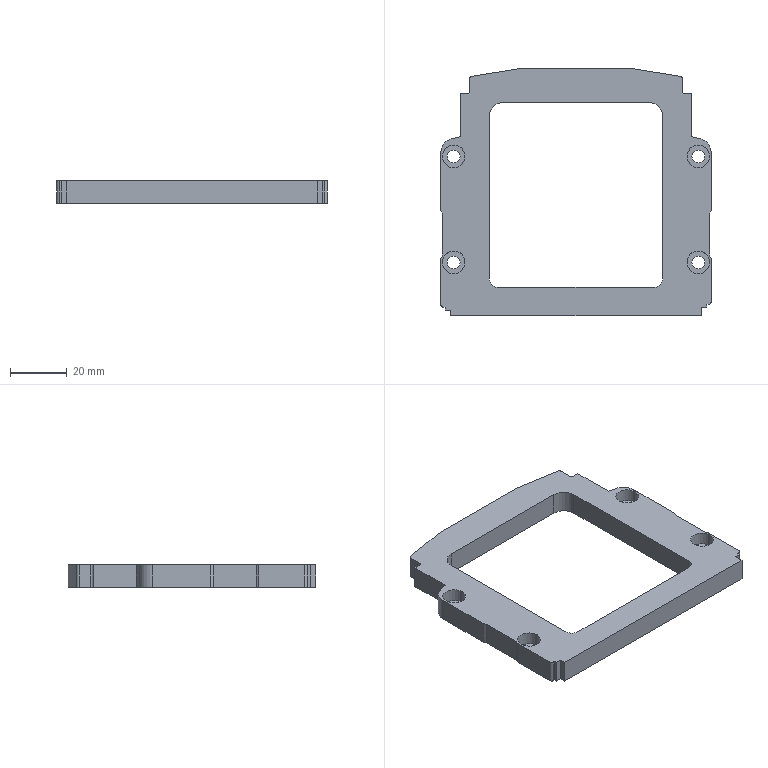Part | NX | 1 solid | 60 faces | box 95 x 87 x 8 mm | volume 29353 mm3 | plane 40 | cylinder 20 | commonest cylinder face diameters 2 x6 4.5 x4 8 x4 10 x4 6 x2